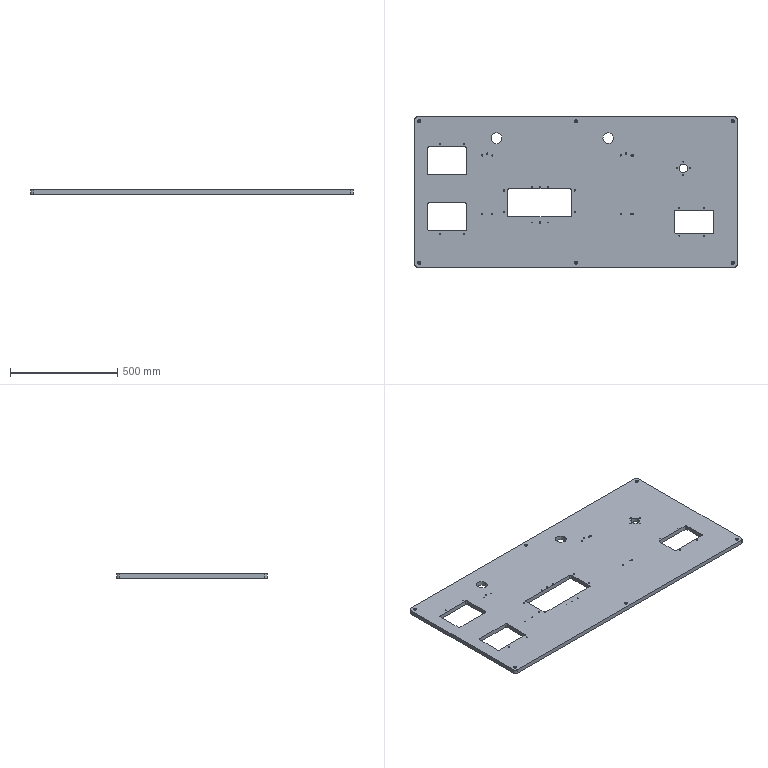Part | STEP file | QA-AD02 | 1 solid | 158 faces | box 1500 x 700 x 20 mm | volume 18757856 mm3 | cylinder 118 | plane 28 | cone 12 | commonest cylinder face diameters 5 x32 4.2 x24 12 x16 6 x12 9 x12 15 x12